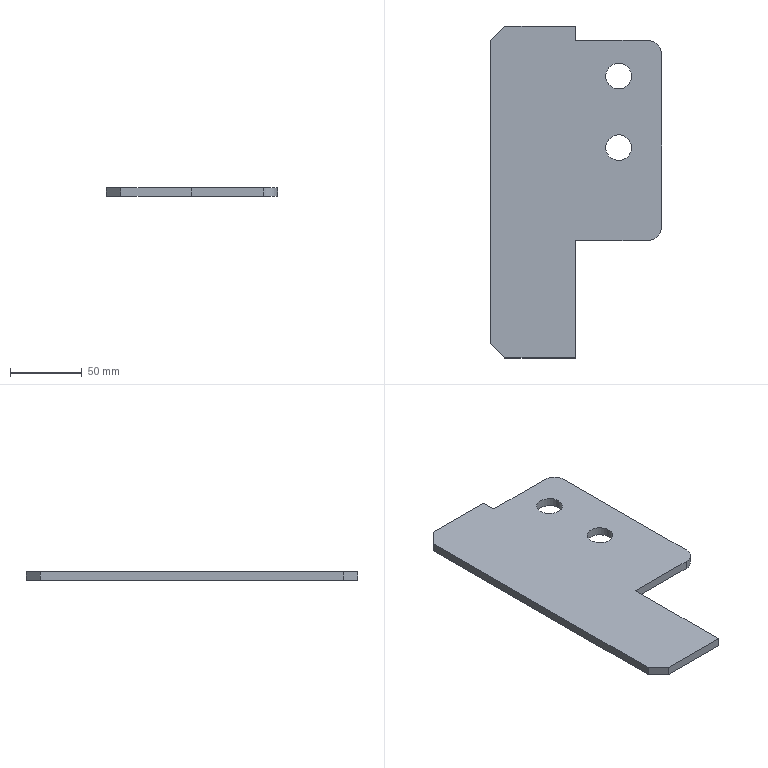Part | STEP file | PN_0034 channel connecting plate_Default<As Machined> | 1 solid | 16 faces | box 119.5 x 232 x 6 mm | volume 129313 mm3 | plane 12 | cylinder 4 | commonest cylinder face diameters 18 x2 20 x2
STEP:
#1=CARTESIAN_POINT('',(0.,0.,0.));
#2=DIRECTION('',(0.,0.,1.));
#3=DIRECTION('',(1.,0.,0.));
#4=AXIS2_PLACEMENT_3D('',#1,#2,#3);
#5=CARTESIAN_POINT('',(-19.75,-116.,6.));
#6=VERTEX_POINT('',#5);
#7=CARTESIAN_POINT('',(-19.75,-116.,0.));
#8=VERTEX_POINT('',#7);
#9=CARTESIAN_POINT('',(-19.75,-116.,6.));
#10=DIRECTION('',(0.,0.,-1.));
#11=VECTOR('',#10,1.);
#12=LINE('',#9,#11);
#13=CARTESIAN_POINT('',(-19.75,-116.,6.));
#14=DIRECTION('',(0.7071,0.7071,0.));
#15=DIRECTION('',(0.,0.,-1.));
#16=AXIS2_PLACEMENT_3D('',#13,#14,#15);
#17=PLANE('',#16);
#18=CARTESIAN_POINT('',(0.,0.));
#19=DIRECTION('',(1.,0.));
#20=VECTOR('',#19,1.);
#21=LINE('',#18,#20);
#22=(GEOMETRIC_REPRESENTATION_CONTEXT(2)PARAMETRIC_REPRESENTATION_CONTEXT()REPRESENTATION_CONTEXT('',''));
#23=DEFINITIONAL_REPRESENTATION('',(#21),#22);
#24=PCURVE('',#17,#23);
#25=CARTESIAN_POINT('',(-29.75,-116.,6.));
#26=DIRECTION('',(0.,1.,0.));
#27=DIRECTION('',(0.,0.,1.));
#28=AXIS2_PLACEMENT_3D('',#25,#26,#27);
#29=PLANE('',#28);
#30=CARTESIAN_POINT('',(0.,10.));
#31=DIRECTION('',(-1.,0.));
#32=VECTOR('',#31,1.);
#33=LINE('',#30,#32);
#34=(GEOMETRIC_REPRESENTATION_CONTEXT(2)PARAMETRIC_REPRESENTATION_CONTEXT()REPRESENTATION_CONTEXT('',''));
#35=DEFINITIONAL_REPRESENTATION('',(#33),#34);
#36=PCURVE('',#29,#35);
#37=SURFACE_CURVE('',#12,(#24,#36),.PCURVE_S1.);
#38=EDGE_CURVE('',#6,#8,#37,.T.);
#39=ORIENTED_EDGE('',*,*,#38,.F.);
#40=CARTESIAN_POINT('',(-29.75,-106.,6.));
#41=VERTEX_POINT('',#40);
#42=CARTESIAN_POINT('',(-67.875,-67.875,6.));
#43=DIRECTION('',(0.7071,-0.7071,0.));
#44=VECTOR('',#43,1.);
#45=LINE('',#42,#44);
#46=CARTESIAN_POINT('',(0.,68.059));
#47=DIRECTION('',(0.,-1.));
#48=VECTOR('',#47,1.);
#49=LINE('',#46,#48);
#50=(GEOMETRIC_REPRESENTATION_CONTEXT(2)PARAMETRIC_REPRESENTATION_CONTEXT()REPRESENTATION_CONTEXT('',''));
#51=DEFINITIONAL_REPRESENTATION('',(#49),#50);
#52=PCURVE('',#17,#51);
#53=CARTESIAN_POINT('',(0.,0.,6.));
#54=DIRECTION('',(0.,0.,1.));
#55=DIRECTION('',(1.,0.,0.));
#56=AXIS2_PLACEMENT_3D('',#53,#54,#55);
#57=PLANE('',#56);
#58=CARTESIAN_POINT('',(-67.875,-67.875));
#59=DIRECTION('',(0.7071,-0.7071));
#60=VECTOR('',#59,1.);
#61=LINE('',#58,#60);
#62=(GEOMETRIC_REPRESENTATION_CONTEXT(2)PARAMETRIC_REPRESENTATION_CONTEXT()REPRESENTATION_CONTEXT('',''));
#63=DEFINITIONAL_REPRESENTATION('',(#61),#62);
#64=PCURVE('',#57,#63);
#65=SURFACE_CURVE('',#45,(#52,#64),.PCURVE_S1.);
#66=EDGE_CURVE('',#41,#6,#65,.T.);
#67=ORIENTED_EDGE('',*,*,#66,.F.);
#68=CARTESIAN_POINT('',(-29.75,-106.,0.));
#69=VERTEX_POINT('',#68);
#70=CARTESIAN_POINT('',(-29.75,-106.,6.));
#71=DIRECTION('',(0.,0.,1.));
#72=VECTOR('',#71,1.);
#73=LINE('',#70,#72);
#74=CARTESIAN_POINT('',(0.,14.142));
#75=DIRECTION('',(-1.,0.));
#76=VECTOR('',#75,1.);
#77=LINE('',#74,#76);
#78=(GEOMETRIC_REPRESENTATION_CONTEXT(2)PARAMETRIC_REPRESENTATION_CONTEXT()REPRESENTATION_CONTEXT('',''));
#79=DEFINITIONAL_REPRESENTATION('',(#77),#78);
#80=PCURVE('',#17,#79);
#81=CARTESIAN_POINT('',(-29.75,116.,6.));
#82=DIRECTION('',(1.,0.,0.));
#83=DIRECTION('',(0.,0.,-1.));
#84=AXIS2_PLACEMENT_3D('',#81,#82,#83);
#85=PLANE('',#84);
#86=CARTESIAN_POINT('',(0.,-222.));
#87=DIRECTION('',(-1.,0.));
#88=VECTOR('',#87,1.);
#89=LINE('',#86,#88);
#90=(GEOMETRIC_REPRESENTATION_CONTEXT(2)PARAMETRIC_REPRESENTATION_CONTEXT()REPRESENTATION_CONTEXT('',''));
#91=DEFINITIONAL_REPRESENTATION('',(#89),#90);
#92=PCURVE('',#85,#91);
#93=SURFACE_CURVE('',#73,(#80,#92),.PCURVE_S1.);
#94=EDGE_CURVE('',#69,#41,#93,.T.);
#95=ORIENTED_EDGE('',*,*,#94,.F.);
#96=CARTESIAN_POINT('',(-19.75,-116.,0.));
#97=DIRECTION('',(-0.7071,0.7071,0.));
#98=VECTOR('',#97,1.);
#99=LINE('',#96,#98);
#100=CARTESIAN_POINT('',(6.,0.));
#101=DIRECTION('',(0.,1.));
#102=VECTOR('',#101,1.);
#103=LINE('',#100,#102);
#104=(GEOMETRIC_REPRESENTATION_CONTEXT(2)PARAMETRIC_REPRESENTATION_CONTEXT()REPRESENTATION_CONTEXT('',''));
#105=DEFINITIONAL_REPRESENTATION('',(#103),#104);
#106=PCURVE('',#17,#105);
#107=CARTESIAN_POINT('',(0.,0.,0.));
#108=DIRECTION('',(0.,0.,1.));
#109=DIRECTION('',(1.,0.,0.));
#110=AXIS2_PLACEMENT_3D('',#107,#108,#109);
#111=PLANE('',#110);
#112=CARTESIAN_POINT('',(-19.75,-116.));
#113=DIRECTION('',(-0.7071,0.7071));
#114=VECTOR('',#113,1.);
#115=LINE('',#112,#114);
#116=(GEOMETRIC_REPRESENTATION_CONTEXT(2)PARAMETRIC_REPRESENTATION_CONTEXT()REPRESENTATION_CONTEXT('',''));
#117=DEFINITIONAL_REPRESENTATION('',(#115),#116);
#118=PCURVE('',#111,#117);
#119=SURFACE_CURVE('',#99,(#106,#118),.PCURVE_S1.);
#120=EDGE_CURVE('',#8,#69,#119,.T.);
#121=ORIENTED_EDGE('',*,*,#120,.F.);
#122=EDGE_LOOP('',(#39,#67,#95,#121));
#123=FACE_BOUND('',#122,.T.);
#124=ADVANCED_FACE('',(#123),#17,.F.);
#125=CARTESIAN_POINT('',(-19.75,116.,0.));
#126=VERTEX_POINT('',#125);
#127=CARTESIAN_POINT('',(-19.75,116.,6.));
#128=VERTEX_POINT('',#127);
#129=CARTESIAN_POINT('',(-19.75,116.,6.));
#130=DIRECTION('',(0.,0.,1.));
#131=VECTOR('',#130,1.);
#132=LINE('',#129,#131);
#133=CARTESIAN_POINT('',(-19.75,116.,6.));
#134=DIRECTION('',(0.7071,-0.7071,0.));
#135=DIRECTION('',(0.,0.,1.));
#136=AXIS2_PLACEMENT_3D('',#133,#134,#135);
#137=PLANE('',#136);
#138=CARTESIAN_POINT('',(0.,0.));
#139=DIRECTION('',(1.,0.));
#140=VECTOR('',#139,1.);
#141=LINE('',#138,#140);
#142=(GEOMETRIC_REPRESENTATION_CONTEXT(2)PARAMETRIC_REPRESENTATION_CONTEXT()REPRESENTATION_CONTEXT('',''));
#143=DEFINITIONAL_REPRESENTATION('',(#141),#142);
#144=PCURVE('',#137,#143);
#145=CARTESIAN_POINT('',(-29.75,116.,6.));
#146=DIRECTION('',(0.,-1.,0.));
#147=DIRECTION('',(0.,0.,-1.));
#148=AXIS2_PLACEMENT_3D('',#145,#146,#147);
#149=PLANE('',#148);
#150=CARTESIAN_POINT('',(0.,10.));
#151=DIRECTION('',(-1.,0.));
#152=VECTOR('',#151,1.);
#153=LINE('',#150,#152);
#154=(GEOMETRIC_REPRESENTATION_CONTEXT(2)PARAMETRIC_REPRESENTATION_CONTEXT()REPRESENTATION_CONTEXT('',''));
#155=DEFINITIONAL_REPRESENTATION('',(#153),#154);
#156=PCURVE('',#149,#155);
#157=SURFACE_CURVE('',#132,(#144,#156),.PCURVE_S1.);
#158=EDGE_CURVE('',#126,#128,#157,.T.);
#159=ORIENTED_EDGE('',*,*,#158,.F.);
#160=CARTESIAN_POINT('',(-29.75,106.,0.));
#161=VERTEX_POINT('',#160);
#162=CARTESIAN_POINT('',(-19.75,116.,0.));
#163=DIRECTION('',(0.7071,0.7071,0.));
#164=VECTOR('',#163,1.);
#165=LINE('',#162,#164);
#166=CARTESIAN_POINT('',(-6.,0.));
#167=DIRECTION('',(0.,-1.));
#168=VECTOR('',#167,1.);
#169=LINE('',#166,#168);
#170=(GEOMETRIC_REPRESENTATION_CONTEXT(2)PARAMETRIC_REPRESENTATION_CONTEXT()REPRESENTATION_CONTEXT('',''));
#171=DEFINITIONAL_REPRESENTATION('',(#169),#170);
#172=PCURVE('',#137,#171);
#173=CARTESIAN_POINT('',(-19.75,116.));
#174=DIRECTION('',(0.7071,0.7071));
#175=VECTOR('',#174,1.);
#176=LINE('',#173,#175);
#177=(GEOMETRIC_REPRESENTATION_CONTEXT(2)PARAMETRIC_REPRESENTATION_CONTEXT()REPRESENTATION_CONTEXT('',''));
#178=DEFINITIONAL_REPRESENTATION('',(#176),#177);
#179=PCURVE('',#111,#178);
#180=SURFACE_CURVE('',#165,(#172,#179),.PCURVE_S1.);
#181=EDGE_CURVE('',#161,#126,#180,.T.);
#182=ORIENTED_EDGE('',*,*,#181,.F.);
#183=CARTESIAN_POINT('',(-29.75,106.,6.));
#184=VERTEX_POINT('',#183);
#185=CARTESIAN_POINT('',(-29.75,106.,6.));
#186=DIRECTION('',(0.,0.,-1.));
#187=VECTOR('',#186,1.);
#188=LINE('',#185,#187);
#189=CARTESIAN_POINT('',(0.,14.142));
#190=DIRECTION('',(-1.,0.));
#191=VECTOR('',#190,1.);
#192=LINE('',#189,#191);
#193=(GEOMETRIC_REPRESENTATION_CONTEXT(2)PARAMETRIC_REPRESENTATION_CONTEXT()REPRESENTATION_CONTEXT('',''));
#194=DEFINITIONAL_REPRESENTATION('',(#192),#193);
#195=PCURVE('',#137,#194);
#196=CARTESIAN_POINT('',(0.,-10.));
#197=DIRECTION('',(1.,0.));
#198=VECTOR('',#197,1.);
#199=LINE('',#196,#198);
#200=(GEOMETRIC_REPRESENTATION_CONTEXT(2)PARAMETRIC_REPRESENTATION_CONTEXT()REPRESENTATION_CONTEXT('',''));
#201=DEFINITIONAL_REPRESENTATION('',(#199),#200);
#202=PCURVE('',#85,#201);
#203=SURFACE_CURVE('',#188,(#195,#202),.PCURVE_S1.);
#204=EDGE_CURVE('',#184,#161,#203,.T.);
#205=ORIENTED_EDGE('',*,*,#204,.F.);
#206=CARTESIAN_POINT('',(-67.875,67.875,6.));
#207=DIRECTION('',(-0.7071,-0.7071,0.));
#208=VECTOR('',#207,1.);
#209=LINE('',#206,#208);
#210=CARTESIAN_POINT('',(0.,68.059));
#211=DIRECTION('',(0.,1.));
#212=VECTOR('',#211,1.);
#213=LINE('',#210,#212);
#214=(GEOMETRIC_REPRESENTATION_CONTEXT(2)PARAMETRIC_REPRESENTATION_CONTEXT()REPRESENTATION_CONTEXT('',''));
#215=DEFINITIONAL_REPRESENTATION('',(#213),#214);
#216=PCURVE('',#137,#215);
#217=CARTESIAN_POINT('',(-67.875,67.875));
#218=DIRECTION('',(-0.7071,-0.7071));
#219=VECTOR('',#218,1.);
#220=LINE('',#217,#219);
#221=(GEOMETRIC_REPRESENTATION_CONTEXT(2)PARAMETRIC_REPRESENTATION_CONTEXT()REPRESENTATION_CONTEXT('',''));
#222=DEFINITIONAL_REPRESENTATION('',(#220),#221);
#223=PCURVE('',#57,#222);
#224=SURFACE_CURVE('',#209,(#216,#223),.PCURVE_S1.);
#225=EDGE_CURVE('',#128,#184,#224,.T.);
#226=ORIENTED_EDGE('',*,*,#225,.F.);
#227=EDGE_LOOP('',(#159,#182,#205,#226));
#228=FACE_BOUND('',#227,.T.);
#229=ADVANCED_FACE('',(#228),#137,.F.);
#230=CARTESIAN_POINT('',(29.75,-116.,0.));
#231=VERTEX_POINT('',#230);
#232=CARTESIAN_POINT('',(29.75,-34.,0.));
#233=VERTEX_POINT('',#232);
#234=CARTESIAN_POINT('',(29.75,-34.,0.));
#235=DIRECTION('',(0.,1.,0.));
#236=VECTOR('',#235,1.);
#237=LINE('',#234,#236);
#238=CARTESIAN_POINT('',(29.75,-34.,6.));
#239=DIRECTION('',(-1.,0.,0.));
#240=DIRECTION('',(0.,-1.,0.));
#241=AXIS2_PLACEMENT_3D('',#238,#239,#240);
#242=PLANE('',#241);
#243=CARTESIAN_POINT('',(0.,-6.));
#244=DIRECTION('',(-1.,0.));
#245=VECTOR('',#244,1.);
#246=LINE('',#243,#245);
#247=(GEOMETRIC_REPRESENTATION_CONTEXT(2)PARAMETRIC_REPRESENTATION_CONTEXT()REPRESENTATION_CONTEXT('',''));
#248=DEFINITIONAL_REPRESENTATION('',(#246),#247);
#249=PCURVE('',#242,#248);
#250=CARTESIAN_POINT('',(29.75,-34.));
#251=DIRECTION('',(0.,1.));
#252=VECTOR('',#251,1.);
#253=LINE('',#250,#252);
#254=(GEOMETRIC_REPRESENTATION_CONTEXT(2)PARAMETRIC_REPRESENTATION_CONTEXT()REPRESENTATION_CONTEXT('',''));
#255=DEFINITIONAL_REPRESENTATION('',(#253),#254);
#256=PCURVE('',#111,#255);
#257=SURFACE_CURVE('',#237,(#249,#256),.PCURVE_S1.);
#258=EDGE_CURVE('',#231,#233,#257,.T.);
#259=ORIENTED_EDGE('',*,*,#258,.T.);
#260=CARTESIAN_POINT('',(29.75,-34.,6.));
#261=VERTEX_POINT('',#260);
#262=CARTESIAN_POINT('',(29.75,-34.,6.));
#263=DIRECTION('',(0.,0.,-1.));
#264=VECTOR('',#263,1.);
#265=LINE('',#262,#264);
#266=CARTESIAN_POINT('',(0.,0.));
#267=DIRECTION('',(0.,-1.));
#268=VECTOR('',#267,1.);
#269=LINE('',#266,#268);
#270=(GEOMETRIC_REPRESENTATION_CONTEXT(2)PARAMETRIC_REPRESENTATION_CONTEXT()REPRESENTATION_CONTEXT('',''));
#271=DEFINITIONAL_REPRESENTATION('',(#269),#270);
#272=PCURVE('',#242,#271);
#273=CARTESIAN_POINT('',(89.75,-34.,6.));
#274=DIRECTION('',(0.,1.,0.));
#275=DIRECTION('',(-1.,0.,0.));
#276=AXIS2_PLACEMENT_3D('',#273,#274,#275);
#277=PLANE('',#276);
#278=CARTESIAN_POINT('',(60.,0.));
#279=DIRECTION('',(0.,-1.));
#280=VECTOR('',#279,1.);
#281=LINE('',#278,#280);
#282=(GEOMETRIC_REPRESENTATION_CONTEXT(2)PARAMETRIC_REPRESENTATION_CONTEXT()REPRESENTATION_CONTEXT('',''));
#283=DEFINITIONAL_REPRESENTATION('',(#281),#282);
#284=PCURVE('',#277,#283);
#285=SURFACE_CURVE('',#265,(#272,#284),.PCURVE_S1.);
#286=EDGE_CURVE('',#261,#233,#285,.T.);
#287=ORIENTED_EDGE('',*,*,#286,.F.);
#288=CARTESIAN_POINT('',(29.75,-116.,6.));
#289=VERTEX_POINT('',#288);
#290=CARTESIAN_POINT('',(29.75,-34.,6.));
#291=DIRECTION('',(0.,1.,0.));
#292=VECTOR('',#291,1.);
#293=LINE('',#290,#292);
#294=CARTESIAN_POINT('',(0.,0.));
#295=DIRECTION('',(-1.,0.));
#296=VECTOR('',#295,1.);
#297=LINE('',#294,#296);
#298=(GEOMETRIC_REPRESENTATION_CONTEXT(2)PARAMETRIC_REPRESENTATION_CONTEXT()REPRESENTATION_CONTEXT('',''));
#299=DEFINITIONAL_REPRESENTATION('',(#297),#298);
#300=PCURVE('',#242,#299);
#301=CARTESIAN_POINT('',(29.75,-34.));
#302=DIRECTION('',(0.,1.));
#303=VECTOR('',#302,1.);
#304=LINE('',#301,#303);
#305=(GEOMETRIC_REPRESENTATION_CONTEXT(2)PARAMETRIC_REPRESENTATION_CONTEXT()REPRESENTATION_CONTEXT('',''));
#306=DEFINITIONAL_REPRESENTATION('',(#304),#305);
#307=PCURVE('',#57,#306);
#308=SURFACE_CURVE('',#293,(#300,#307),.PCURVE_S1.);
#309=EDGE_CURVE('',#289,#261,#308,.T.);
#310=ORIENTED_EDGE('',*,*,#309,.F.);
#311=CARTESIAN_POINT('',(29.75,-116.,6.));
#312=DIRECTION('',(0.,0.,-1.));
#313=VECTOR('',#312,1.);
#314=LINE('',#311,#313);
#315=CARTESIAN_POINT('',(82.,0.));
#316=DIRECTION('',(0.,-1.));
#317=VECTOR('',#316,1.);
#318=LINE('',#315,#317);
#319=(GEOMETRIC_REPRESENTATION_CONTEXT(2)PARAMETRIC_REPRESENTATION_CONTEXT()REPRESENTATION_CONTEXT('',''));
#320=DEFINITIONAL_REPRESENTATION('',(#318),#319);
#321=PCURVE('',#242,#320);
#322=CARTESIAN_POINT('',(0.,59.5));
#323=DIRECTION('',(-1.,0.));
#324=VECTOR('',#323,1.);
#325=LINE('',#322,#324);
#326=(GEOMETRIC_REPRESENTATION_CONTEXT(2)PARAMETRIC_REPRESENTATION_CONTEXT()REPRESENTATION_CONTEXT('',''));
#327=DEFINITIONAL_REPRESENTATION('',(#325),#326);
#328=PCURVE('',#29,#327);
#329=SURFACE_CURVE('',#314,(#321,#328),.PCURVE_S1.);
#330=EDGE_CURVE('',#289,#231,#329,.T.);
#331=ORIENTED_EDGE('',*,*,#330,.T.);
#332=EDGE_LOOP('',(#259,#287,#310,#331));
#333=FACE_BOUND('',#332,.T.);
#334=ADVANCED_FACE('',(#333),#242,.F.);
#335=CARTESIAN_POINT('',(79.75,-34.,0.));
#336=VERTEX_POINT('',#335);
#337=CARTESIAN_POINT('',(89.75,-34.,0.));
#338=DIRECTION('',(1.,0.,0.));
#339=VECTOR('',#338,1.);
#340=LINE('',#337,#339);
#341=CARTESIAN_POINT('',(0.,-6.));
#342=DIRECTION('',(-1.,0.));
#343=VECTOR('',#342,1.);
#344=LINE('',#341,#343);
#345=(GEOMETRIC_REPRESENTATION_CONTEXT(2)PARAMETRIC_REPRESENTATION_CONTEXT()REPRESENTATION_CONTEXT('',''));
#346=DEFINITIONAL_REPRESENTATION('',(#344),#345);
#347=PCURVE('',#277,#346);
#348=CARTESIAN_POINT('',(89.75,-34.));
#349=DIRECTION('',(1.,0.));
#350=VECTOR('',#349,1.);
#351=LINE('',#348,#350);
#352=(GEOMETRIC_REPRESENTATION_CONTEXT(2)PARAMETRIC_REPRESENTATION_CONTEXT()REPRESENTATION_CONTEXT('',''));
#353=DEFINITIONAL_REPRESENTATION('',(#351),#352);
#354=PCURVE('',#111,#353);
#355=SURFACE_CURVE('',#340,(#347,#354),.PCURVE_S1.);
#356=EDGE_CURVE('',#233,#336,#355,.T.);
#357=ORIENTED_EDGE('',*,*,#356,.T.);
#358=CARTESIAN_POINT('',(79.75,-34.,6.));
#359=VERTEX_POINT('',#358);
#360=CARTESIAN_POINT('',(79.75,-34.,6.));
#361=DIRECTION('',(0.,0.,1.));
#362=VECTOR('',#361,1.);
#363=LINE('',#360,#362);
#364=CARTESIAN_POINT('',(10.,0.));
#365=DIRECTION('',(0.,1.));
#366=VECTOR('',#365,1.);
#367=LINE('',#364,#366);
#368=(GEOMETRIC_REPRESENTATION_CONTEXT(2)PARAMETRIC_REPRESENTATION_CONTEXT()REPRESENTATION_CONTEXT('',''));
#369=DEFINITIONAL_REPRESENTATION('',(#367),#368);
#370=PCURVE('',#277,#369);
#371=CARTESIAN_POINT('',(79.75,-24.,6.));
#372=DIRECTION('',(0.,0.,-1.));
#373=DIRECTION('',(-1.,0.,0.));
#374=AXIS2_PLACEMENT_3D('',#371,#372,#373);
#375=CYLINDRICAL_SURFACE('',#374,10.);
#376=CARTESIAN_POINT('',(4.712,0.));
#377=DIRECTION('',(0.,-1.));
#378=VECTOR('',#377,1.);
#379=LINE('',#376,#378);
#380=(GEOMETRIC_REPRESENTATION_CONTEXT(2)PARAMETRIC_REPRESENTATION_CONTEXT()REPRESENTATION_CONTEXT('',''));
#381=DEFINITIONAL_REPRESENTATION('',(#379),#380);
#382=PCURVE('',#375,#381);
#383=SURFACE_CURVE('',#363,(#370,#382),.PCURVE_S1.);
#384=EDGE_CURVE('',#336,#359,#383,.T.);
#385=ORIENTED_EDGE('',*,*,#384,.T.);
#386=CARTESIAN_POINT('',(89.75,-34.,6.));
#387=DIRECTION('',(1.,0.,0.));
#388=VECTOR('',#387,1.);
#389=LINE('',#386,#388);
#390=CARTESIAN_POINT('',(0.,0.));
#391=DIRECTION('',(-1.,0.));
#392=VECTOR('',#391,1.);
#393=LINE('',#390,#392);
#394=(GEOMETRIC_REPRESENTATION_CONTEXT(2)PARAMETRIC_REPRESENTATION_CONTEXT()REPRESENTATION_CONTEXT('',''));
#395=DEFINITIONAL_REPRESENTATION('',(#393),#394);
#396=PCURVE('',#277,#395);
#397=CARTESIAN_POINT('',(89.75,-34.));
#398=DIRECTION('',(1.,0.));
#399=VECTOR('',#398,1.);
#400=LINE('',#397,#399);
#401=(GEOMETRIC_REPRESENTATION_CONTEXT(2)PARAMETRIC_REPRESENTATION_CONTEXT()REPRESENTATION_CONTEXT('',''));
#402=DEFINITIONAL_REPRESENTATION('',(#400),#401);
#403=PCURVE('',#57,#402);
#404=SURFACE_CURVE('',#389,(#396,#403),.PCURVE_S1.);
#405=EDGE_CURVE('',#261,#359,#404,.T.);
#406=ORIENTED_EDGE('',*,*,#405,.F.);
#407=ORIENTED_EDGE('',*,*,#286,.T.);
#408=EDGE_LOOP('',(#357,#385,#406,#407));
#409=FACE_BOUND('',#408,.T.);
#410=ADVANCED_FACE('',(#409),#277,.F.);
#411=CARTESIAN_POINT('',(89.75,-24.,6.));
#412=VERTEX_POINT('',#411);
#413=CARTESIAN_POINT('',(89.75,96.,6.));
#414=VERTEX_POINT('',#413);
#415=CARTESIAN_POINT('',(89.75,106.,6.));
#416=DIRECTION('',(0.,1.,0.));
#417=VECTOR('',#416,1.);
#418=LINE('',#415,#417);
#419=CARTESIAN_POINT('',(89.75,106.,6.));
#420=DIRECTION('',(-1.,0.,0.));
#421=DIRECTION('',(0.,-1.,0.));
#422=AXIS2_PLACEMENT_3D('',#419,#420,#421);
#423=PLANE('',#422);
#424=CARTESIAN_POINT('',(0.,0.));
#425=DIRECTION('',(-1.,0.));
#426=VECTOR('',#425,1.);
#427=LINE('',#424,#426);
#428=(GEOMETRIC_REPRESENTATION_CONTEXT(2)PARAMETRIC_REPRESENTATION_CONTEXT()REPRESENTATION_CONTEXT('',''));
#429=DEFINITIONAL_REPRESENTATION('',(#427),#428);
#430=PCURVE('',#423,#429);
#431=CARTESIAN_POINT('',(89.75,106.));
#432=DIRECTION('',(0.,1.));
#433=VECTOR('',#432,1.);
#434=LINE('',#431,#433);
#435=(GEOMETRIC_REPRESENTATION_CONTEXT(2)PARAMETRIC_REPRESENTATION_CONTEXT()REPRESENTATION_CONTEXT('',''));
#436=DEFINITIONAL_REPRESENTATION('',(#434),#435);
#437=PCURVE('',#57,#436);
#438=SURFACE_CURVE('',#418,(#430,#437),.PCURVE_S1.);
#439=EDGE_CURVE('',#412,#414,#438,.T.);
#440=ORIENTED_EDGE('',*,*,#439,.F.);
#441=CARTESIAN_POINT('',(89.75,-24.,0.));
#442=VERTEX_POINT('',#441);
#443=CARTESIAN_POINT('',(89.75,-24.,6.));
#444=DIRECTION('',(0.,0.,-1.));
#445=VECTOR('',#444,1.);
#446=LINE('',#443,#445);
#447=CARTESIAN_POINT('',(130.,0.));
#448=DIRECTION('',(0.,-1.));
#449=VECTOR('',#448,1.);
#450=LINE('',#447,#449);
#451=(GEOMETRIC_REPRESENTATION_CONTEXT(2)PARAMETRIC_REPRESENTATION_CONTEXT()REPRESENTATION_CONTEXT('',''));
#452=DEFINITIONAL_REPRESENTATION('',(#450),#451);
#453=PCURVE('',#423,#452);
#454=CARTESIAN_POINT('',(3.142,0.));
#455=DIRECTION('',(0.,1.));
#456=VECTOR('',#455,1.);
#457=LINE('',#454,#456);
#458=(GEOMETRIC_REPRESENTATION_CONTEXT(2)PARAMETRIC_REPRESENTATION_CONTEXT()REPRESENTATION_CONTEXT('',''));
#459=DEFINITIONAL_REPRESENTATION('',(#457),#458);
#460=PCURVE('',#375,#459);
#461=SURFACE_CURVE('',#446,(#453,#460),.PCURVE_S1.);
#462=EDGE_CURVE('',#412,#442,#461,.T.);
#463=ORIENTED_EDGE('',*,*,#462,.T.);
#464=CARTESIAN_POINT('',(89.75,96.,0.));
#465=VERTEX_POINT('',#464);
#466=CARTESIAN_POINT('',(89.75,106.,0.));
#467=DIRECTION('',(0.,1.,0.));
#468=VECTOR('',#467,1.);
#469=LINE('',#466,#468);
#470=CARTESIAN_POINT('',(0.,-6.));
#471=DIRECTION('',(-1.,0.));
#472=VECTOR('',#471,1.);
#473=LINE('',#470,#472);
#474=(GEOMETRIC_REPRESENTATION_CONTEXT(2)PARAMETRIC_REPRESENTATION_CONTEXT()REPRESENTATION_CONTEXT('',''));
#475=DEFINITIONAL_REPRESENTATION('',(#473),#474);
#476=PCURVE('',#423,#475);
#477=CARTESIAN_POINT('',(89.75,106.));
#478=DIRECTION('',(0.,1.));
#479=VECTOR('',#478,1.);
#480=LINE('',#477,#479);
#481=(GEOMETRIC_REPRESENTATION_CONTEXT(2)PARAMETRIC_REPRESENTATION_CONTEXT()REPRESENTATION_CONTEXT('',''));
#482=DEFINITIONAL_REPRESENTATION('',(#480),#481);
#483=PCURVE('',#111,#482);
#484=SURFACE_CURVE('',#469,(#476,#483),.PCURVE_S1.);
#485=EDGE_CURVE('',#442,#465,#484,.T.);
#486=ORIENTED_EDGE('',*,*,#485,.T.);
#487=CARTESIAN_POINT('',(89.75,96.,6.));
#488=DIRECTION('',(0.,0.,1.));
#489=VECTOR('',#488,1.);
#490=LINE('',#487,#489);
#491=CARTESIAN_POINT('',(10.,0.));
#492=DIRECTION('',(0.,1.));
#493=VECTOR('',#492,1.);
#494=LINE('',#491,#493);
#495=(GEOMETRIC_REPRESENTATION_CONTEXT(2)PARAMETRIC_REPRESENTATION_CONTEXT()REPRESENTATION_CONTEXT('',''));
#496=DEFINITIONAL_REPRESENTATION('',(#494),#495);
#497=PCURVE('',#423,#496);
#498=CARTESIAN_POINT('',(79.75,96.,6.));
#499=DIRECTION('',(0.,0.,-1.));
#500=DIRECTION('',(-1.,0.,0.));
#501=AXIS2_PLACEMENT_3D('',#498,#499,#500);
#502=CYLINDRICAL_SURFACE('',#501,10.);
#503=CARTESIAN_POINT('',(3.142,0.));
#504=DIRECTION('',(0.,-1.));
#505=VECTOR('',#504,1.);
#506=LINE('',#503,#505);
#507=(GEOMETRIC_REPRESENTATION_CONTEXT(2)PARAMETRIC_REPRESENTATION_CONTEXT()REPRESENTATION_CONTEXT('',''));
#508=DEFINITIONAL_REPRESENTATION('',(#506),#507);
#509=PCURVE('',#502,#508);
#510=SURFACE_CURVE('',#490,(#497,#509),.PCURVE_S1.);
#511=EDGE_CURVE('',#465,#414,#510,.T.);
#512=ORIENTED_EDGE('',*,*,#511,.T.);
#513=EDGE_LOOP('',(#440,#463,#486,#512));
#514=FACE_BOUND('',#513,.T.);
#515=ADVANCED_FACE('',(#514),#423,.F.);
#516=CARTESIAN_POINT('',(79.75,106.,6.));
#517=VERTEX_POINT('',#516);
#518=CARTESIAN_POINT('',(29.75,106.,6.));
#519=VERTEX_POINT('',#518);
#520=CARTESIAN_POINT('',(29.75,106.,6.));
#521=DIRECTION('',(-1.,0.,0.));
#522=VECTOR('',#521,1.);
#523=LINE('',#520,#522);
#524=CARTESIAN_POINT('',(29.75,106.,6.));
#525=DIRECTION('',(0.,-1.,0.));
#526=DIRECTION('',(0.,0.,-1.));
#527=AXIS2_PLACEMENT_3D('',#524,#525,#526);
#528=PLANE('',#527);
#529=CARTESIAN_POINT('',(0.,0.));
#530=DIRECTION('',(0.,-1.));
#531=VECTOR('',#530,1.);
#532=LINE('',#529,#531);
#533=(GEOMETRIC_REPRESENTATION_CONTEXT(2)PARAMETRIC_REPRESENTATION_CONTEXT()REPRESENTATION_CONTEXT('',''));
#534=DEFINITIONAL_REPRESENTATION('',(#532),#533);
#535=PCURVE('',#528,#534);
#536=CARTESIAN_POINT('',(29.75,106.));
#537=DIRECTION('',(-1.,0.));
#538=VECTOR('',#537,1.);
#539=LINE('',#536,#538);
#540=(GEOMETRIC_REPRESENTATION_CONTEXT(2)PARAMETRIC_REPRESENTATION_CONTEXT()REPRESENTATION_CONTEXT('',''));
#541=DEFINITIONAL_REPRESENTATION('',(#539),#540);
#542=PCURVE('',#57,#541);
#543=SURFACE_CURVE('',#523,(#535,#542),.PCURVE_S1.);
#544=EDGE_CURVE('',#517,#519,#543,.T.);
#545=ORIENTED_EDGE('',*,*,#544,.F.);
#546=CARTESIAN_POINT('',(79.75,106.,0.));
#547=VERTEX_POINT('',#546);
#548=CARTESIAN_POINT('',(79.75,106.,6.));
#549=DIRECTION('',(0.,0.,-1.));
#550=VECTOR('',#549,1.);
#551=LINE('',#548,#550);
#552=CARTESIAN_POINT('',(0.,50.));
#553=DIRECTION('',(1.,0.));
#554=VECTOR('',#553,1.);
#555=LINE('',#552,#554);
#556=(GEOMETRIC_REPRESENTATION_CONTEXT(2)PARAMETRIC_REPRESENTATION_CONTEXT()REPRESENTATION_CONTEXT('',''));
#557=DEFINITIONAL_REPRESENTATION('',(#555),#556);
#558=PCURVE('',#528,#557);
#559=CARTESIAN_POINT('',(1.571,0.));
#560=DIRECTION('',(0.,1.));
#561=VECTOR('',#560,1.);
#562=LINE('',#559,#561);
#563=(GEOMETRIC_REPRESENTATION_CONTEXT(2)PARAMETRIC_REPRESENTATION_CONTEXT()REPRESENTATION_CONTEXT('',''));
#564=DEFINITIONAL_REPRESENTATION('',(#562),#563);
#565=PCURVE('',#502,#564);
#566=SURFACE_CURVE('',#551,(#558,#565),.PCURVE_S1.);
#567=EDGE_CURVE('',#517,#547,#566,.T.);
#568=ORIENTED_EDGE('',*,*,#567,.T.);
#569=CARTESIAN_POINT('',(29.75,106.,0.));
#570=VERTEX_POINT('',#569);
#571=CARTESIAN_POINT('',(29.75,106.,0.));
#572=DIRECTION('',(-1.,0.,0.));
#573=VECTOR('',#572,1.);
#574=LINE('',#571,#573);
#575=CARTESIAN_POINT('',(6.,0.));
#576=DIRECTION('',(0.,-1.));
#577=VECTOR('',#576,1.);
#578=LINE('',#575,#577);
#579=(GEOMETRIC_REPRESENTATION_CONTEXT(2)PARAMETRIC_REPRESENTATION_CONTEXT()REPRESENTATION_CONTEXT('',''));
#580=DEFINITIONAL_REPRESENTATION('',(#578),#579);
#581=PCURVE('',#528,#580);
#582=CARTESIAN_POINT('',(29.75,106.));
#583=DIRECTION('',(-1.,0.));
#584=VECTOR('',#583,1.);
#585=LINE('',#582,#584);
#586=(GEOMETRIC_REPRESENTATION_CONTEXT(2)PARAMETRIC_REPRESENTATION_CONTEXT()REPRESENTATION_CONTEXT('',''));
#587=DEFINITIONAL_REPRESENTATION('',(#585),#586);
#588=PCURVE('',#111,#587);
#589=SURFACE_CURVE('',#574,(#581,#588),.PCURVE_S1.);
#590=EDGE_CURVE('',#547,#570,#589,.T.);
#591=ORIENTED_EDGE('',*,*,#590,.T.);
#592=CARTESIAN_POINT('',(29.75,106.,6.));
#593=DIRECTION('',(0.,0.,-1.));
#594=VECTOR('',#593,1.);
#595=LINE('',#592,#594);
#596=CARTESIAN_POINT('',(0.,0.));
#597=DIRECTION('',(1.,0.));
#598=VECTOR('',#597,1.);
#599=LINE('',#596,#598);
#600=(GEOMETRIC_REPRESENTATION_CONTEXT(2)PARAMETRIC_REPRESENTATION_CONTEXT()REPRESENTATION_CONTEXT('',''));
#601=DEFINITIONAL_REPRESENTATION('',(#599),#600);
#602=PCURVE('',#528,#601);
#603=CARTESIAN_POINT('',(29.75,116.,6.));
#604=DIRECTION('',(-1.,0.,0.));
#605=DIRECTION('',(0.,0.,1.));
#606=AXIS2_PLACEMENT_3D('',#603,#604,#605);
#607=PLANE('',#606);
#608=CARTESIAN_POINT('',(0.,-10.));
#609=DIRECTION('',(-1.,0.));
#610=VECTOR('',#609,1.);
#611=LINE('',#608,#610);
#612=(GEOMETRIC_REPRESENTATION_CONTEXT(2)PARAMETRIC_REPRESENTATION_CONTEXT()REPRESENTATION_CONTEXT('',''));
#613=DEFINITIONAL_REPRESENTATION('',(#611),#612);
#614=PCURVE('',#607,#613);
#615=SURFACE_CURVE('',#595,(#602,#614),.PCURVE_S1.);
#616=EDGE_CURVE('',#519,#570,#615,.T.);
#617=ORIENTED_EDGE('',*,*,#616,.F.);
#618=EDGE_LOOP('',(#545,#568,#591,#617));
#619=FACE_BOUND('',#618,.T.);
#620=ADVANCED_FACE('',(#619),#528,.F.);
#621=CARTESIAN_POINT('',(29.75,116.,0.));
#622=VERTEX_POINT('',#621);
#623=CARTESIAN_POINT('',(29.75,116.,0.));
#624=DIRECTION('',(0.,1.,0.));
#625=VECTOR('',#624,1.);
#626=LINE('',#623,#625);
#627=CARTESIAN_POINT('',(-6.,0.));
#628=DIRECTION('',(0.,1.));
#629=VECTOR('',#628,1.);
#630=LINE('',#627,#629);
#631=(GEOMETRIC_REPRESENTATION_CONTEXT(2)PARAMETRIC_REPRESENTATION_CONTEXT()REPRESENTATION_CONTEXT('',''));
#632=DEFINITIONAL_REPRESENTATION('',(#630),#631);
#633=PCURVE('',#607,#632);
#634=CARTESIAN_POINT('',(29.75,116.));
#635=DIRECTION('',(0.,1.));
#636=VECTOR('',#635,1.);
#637=LINE('',#634,#636);
#638=(GEOMETRIC_REPRESENTATION_CONTEXT(2)PARAMETRIC_REPRESENTATION_CONTEXT()REPRESENTATION_CONTEXT('',''));
#639=DEFINITIONAL_REPRESENTATION('',(#637),#638);
#640=PCURVE('',#111,#639);
#641=SURFACE_CURVE('',#626,(#633,#640),.PCURVE_S1.);
#642=EDGE_CURVE('',#570,#622,#641,.T.);
#643=ORIENTED_EDGE('',*,*,#642,.T.);
#644=CARTESIAN_POINT('',(29.75,116.,6.));
#645=VERTEX_POINT('',#644);
#646=CARTESIAN_POINT('',(29.75,116.,6.));
#647=DIRECTION('',(0.,0.,-1.));
#648=VECTOR('',#647,1.);
#649=LINE('',#646,#648);
#650=CARTESIAN_POINT('',(0.,0.));
#651=DIRECTION('',(-1.,0.));
#652=VECTOR('',#651,1.);
#653=LINE('',#650,#652);
#654=(GEOMETRIC_REPRESENTATION_CONTEXT(2)PARAMETRIC_REPRESENTATION_CONTEXT()REPRESENTATION_CONTEXT('',''));
#655=DEFINITIONAL_REPRESENTATION('',(#653),#654);
#656=PCURVE('',#607,#655);
#657=CARTESIAN_POINT('',(0.,59.5));
#658=DIRECTION('',(1.,0.));
#659=VECTOR('',#658,1.);
#660=LINE('',#657,#659);
#661=(GEOMETRIC_REPRESENTATION_CONTEXT(2)PARAMETRIC_REPRESENTATION_CONTEXT()REPRESENTATION_CONTEXT('',''));
#662=DEFINITIONAL_REPRESENTATION('',(#660),#661);
#663=PCURVE('',#149,#662);
#664=SURFACE_CURVE('',#649,(#656,#663),.PCURVE_S1.);
#665=EDGE_CURVE('',#645,#622,#664,.T.);
#666=ORIENTED_EDGE('',*,*,#665,.F.);
#667=CARTESIAN_POINT('',(29.75,116.,6.));
#668=DIRECTION('',(0.,1.,0.));
#669=VECTOR('',#668,1.);
#670=LINE('',#667,#669);
#671=CARTESIAN_POINT('',(0.,0.));
#672=DIRECTION('',(0.,1.));
#673=VECTOR('',#672,1.);
#674=LINE('',#671,#673);
#675=(GEOMETRIC_REPRESENTATION_CONTEXT(2)PARAMETRIC_REPRESENTATION_CONTEXT()REPRESENTATION_CONTEXT('',''));
#676=DEFINITIONAL_REPRESENTATION('',(#674),#675);
#677=PCURVE('',#607,#676);
#678=CARTESIAN_POINT('',(29.75,116.));
#679=DIRECTION('',(0.,1.));
#680=VECTOR('',#679,1.);
#681=LINE('',#678,#680);
#682=(GEOMETRIC_REPRESENTATION_CONTEXT(2)PARAMETRIC_REPRESENTATION_CONTEXT()REPRESENTATION_CONTEXT('',''));
#683=DEFINITIONAL_REPRESENTATION('',(#681),#682);
#684=PCURVE('',#57,#683);
#685=SURFACE_CURVE('',#670,(#677,#684),.PCURVE_S1.);
#686=EDGE_CURVE('',#519,#645,#685,.T.);
#687=ORIENTED_EDGE('',*,*,#686,.F.);
#688=ORIENTED_EDGE('',*,*,#616,.T.);
#689=EDGE_LOOP('',(#643,#666,#687,#688));
#690=FACE_BOUND('',#689,.T.);
#691=ADVANCED_FACE('',(#690),#607,.F.);
#692=CARTESIAN_POINT('',(-29.75,116.,0.));
#693=DIRECTION('',(-1.,0.,0.));
#694=VECTOR('',#693,1.);
#695=LINE('',#692,#694);
#696=CARTESIAN_POINT('',(6.,0.));
#697=DIRECTION('',(0.,-1.));
#698=VECTOR('',#697,1.);
#699=LINE('',#696,#698);
#700=(GEOMETRIC_REPRESENTATION_CONTEXT(2)PARAMETRIC_REPRESENTATION_CONTEXT()REPRESENTATION_CONTEXT('',''));
#701=DEFINITIONAL_REPRESENTATION('',(#699),#700);
#702=PCURVE('',#149,#701);
#703=CARTESIAN_POINT('',(-29.75,116.));
#704=DIRECTION('',(-1.,0.));
#705=VECTOR('',#704,1.);
#706=LINE('',#703,#705);
#707=(GEOMETRIC_REPRESENTATION_CONTEXT(2)PARAMETRIC_REPRESENTATION_CONTEXT()REPRESENTATION_CONTEXT('',''));
#708=DEFINITIONAL_REPRESENTATION('',(#706),#707);
#709=PCURVE('',#111,#708);
#710=SURFACE_CURVE('',#695,(#702,#709),.PCURVE_S1.);
#711=EDGE_CURVE('',#622,#126,#710,.T.);
#712=ORIENTED_EDGE('',*,*,#711,.T.);
#713=ORIENTED_EDGE('',*,*,#158,.T.);
#714=CARTESIAN_POINT('',(-29.75,116.,6.));
#715=DIRECTION('',(-1.,0.,0.));
#716=VECTOR('',#715,1.);
#717=LINE('',#714,#716);
#718=CARTESIAN_POINT('',(0.,0.));
#719=DIRECTION('',(0.,-1.));
#720=VECTOR('',#719,1.);
#721=LINE('',#718,#720);
#722=(GEOMETRIC_REPRESENTATION_CONTEXT(2)PARAMETRIC_REPRESENTATION_CONTEXT()REPRESENTATION_CONTEXT('',''));
#723=DEFINITIONAL_REPRESENTATION('',(#721),#722);
#724=PCURVE('',#149,#723);
#725=CARTESIAN_POINT('',(-29.75,116.));
#726=DIRECTION('',(-1.,0.));
#727=VECTOR('',#726,1.);
#728=LINE('',#725,#727);
#729=(GEOMETRIC_REPRESENTATION_CONTEXT(2)PARAMETRIC_REPRESENTATION_CONTEXT()REPRESENTATION_CONTEXT('',''));
#730=DEFINITIONAL_REPRESENTATION('',(#728),#729);
#731=PCURVE('',#57,#730);
#732=SURFACE_CURVE('',#717,(#724,#731),.PCURVE_S1.);
#733=EDGE_CURVE('',#645,#128,#732,.T.);
#734=ORIENTED_EDGE('',*,*,#733,.F.);
#735=ORIENTED_EDGE('',*,*,#665,.T.);
#736=EDGE_LOOP('',(#712,#713,#734,#735));
#737=FACE_BOUND('',#736,.T.);
#738=ADVANCED_FACE('',(#737),#149,.F.);
#739=CARTESIAN_POINT('',(-29.75,116.,0.));
#740=DIRECTION('',(0.,-1.,0.));
#741=VECTOR('',#740,1.);
#742=LINE('',#739,#741);
#743=CARTESIAN_POINT('',(6.,0.));
#744=DIRECTION('',(0.,-1.));
#745=VECTOR('',#744,1.);
#746=LINE('',#743,#745);
#747=(GEOMETRIC_REPRESENTATION_CONTEXT(2)PARAMETRIC_REPRESENTATION_CONTEXT()REPRESENTATION_CONTEXT('',''));
#748=DEFINITIONAL_REPRESENTATION('',(#746),#747);
#749=PCURVE('',#85,#748);
#750=CARTESIAN_POINT('',(-29.75,116.));
#751=DIRECTION('',(0.,-1.));
#752=VECTOR('',#751,1.);
#753=LINE('',#750,#752);
#754=(GEOMETRIC_REPRESENTATION_CONTEXT(2)PARAMETRIC_REPRESENTATION_CONTEXT()REPRESENTATION_CONTEXT('',''));
#755=DEFINITIONAL_REPRESENTATION('',(#753),#754);
#756=PCURVE('',#111,#755);
#757=SURFACE_CURVE('',#742,(#749,#756),.PCURVE_S1.);
#758=EDGE_CURVE('',#161,#69,#757,.T.);
#759=ORIENTED_EDGE('',*,*,#758,.T.);
#760=ORIENTED_EDGE('',*,*,#94,.T.);
#761=CARTESIAN_POINT('',(-29.75,116.,6.));
#762=DIRECTION('',(0.,-1.,0.));
#763=VECTOR('',#762,1.);
#764=LINE('',#761,#763);
#765=CARTESIAN_POINT('',(0.,0.));
#766=DIRECTION('',(0.,-1.));
#767=VECTOR('',#766,1.);
#768=LINE('',#765,#767);
#769=(GEOMETRIC_REPRESENTATION_CONTEXT(2)PARAMETRIC_REPRESENTATION_CONTEXT()REPRESENTATION_CONTEXT('',''));
#770=DEFINITIONAL_REPRESENTATION('',(#768),#769);
#771=PCURVE('',#85,#770);
#772=CARTESIAN_POINT('',(-29.75,116.));
#773=DIRECTION('',(0.,-1.));
#774=VECTOR('',#773,1.);
#775=LINE('',#772,#774);
#776=(GEOMETRIC_REPRESENTATION_CONTEXT(2)PARAMETRIC_REPRESENTATION_CONTEXT()REPRESENTATION_CONTEXT('',''));
#777=DEFINITIONAL_REPRESENTATION('',(#775),#776);
#778=PCURVE('',#57,#777);
#779=SURFACE_CURVE('',#764,(#771,#778),.PCURVE_S1.);
#780=EDGE_CURVE('',#184,#41,#779,.T.);
#781=ORIENTED_EDGE('',*,*,#780,.F.);
#782=ORIENTED_EDGE('',*,*,#204,.T.);
#783=EDGE_LOOP('',(#759,#760,#781,#782));
#784=FACE_BOUND('',#783,.T.);
#785=ADVANCED_FACE('',(#784),#85,.F.);
#786=CARTESIAN_POINT('',(-29.75,-116.,6.));
#787=DIRECTION('',(1.,0.,0.));
#788=VECTOR('',#787,1.);
#789=LINE('',#786,#788);
#790=CARTESIAN_POINT('',(0.,0.));
#791=DIRECTION('',(0.,1.));
#792=VECTOR('',#791,1.);
#793=LINE('',#790,#792);
#794=(GEOMETRIC_REPRESENTATION_CONTEXT(2)PARAMETRIC_REPRESENTATION_CONTEXT()REPRESENTATION_CONTEXT('',''));
#795=DEFINITIONAL_REPRESENTATION('',(#793),#794);
#796=PCURVE('',#29,#795);
#797=CARTESIAN_POINT('',(-29.75,-116.));
#798=DIRECTION('',(1.,0.));
#799=VECTOR('',#798,1.);
#800=LINE('',#797,#799);
#801=(GEOMETRIC_REPRESENTATION_CONTEXT(2)PARAMETRIC_REPRESENTATION_CONTEXT()REPRESENTATION_CONTEXT('',''));
#802=DEFINITIONAL_REPRESENTATION('',(#800),#801);
#803=PCURVE('',#57,#802);
#804=SURFACE_CURVE('',#789,(#796,#803),.PCURVE_S1.);
#805=EDGE_CURVE('',#6,#289,#804,.T.);
#806=ORIENTED_EDGE('',*,*,#805,.F.);
#807=ORIENTED_EDGE('',*,*,#38,.T.);
#808=CARTESIAN_POINT('',(-29.75,-116.,0.));
#809=DIRECTION('',(1.,0.,0.));
#810=VECTOR('',#809,1.);
#811=LINE('',#808,#810);
#812=CARTESIAN_POINT('',(-6.,0.));
#813=DIRECTION('',(0.,1.));
#814=VECTOR('',#813,1.);
#815=LINE('',#812,#814);
#816=(GEOMETRIC_REPRESENTATION_CONTEXT(2)PARAMETRIC_REPRESENTATION_CONTEXT()REPRESENTATION_CONTEXT('',''));
#817=DEFINITIONAL_REPRESENTATION('',(#815),#816);
#818=PCURVE('',#29,#817);
#819=CARTESIAN_POINT('',(-29.75,-116.));
#820=DIRECTION('',(1.,0.));
#821=VECTOR('',#820,1.);
#822=LINE('',#819,#821);
#823=(GEOMETRIC_REPRESENTATION_CONTEXT(2)PARAMETRIC_REPRESENTATION_CONTEXT()REPRESENTATION_CONTEXT('',''));
#824=DEFINITIONAL_REPRESENTATION('',(#822),#823);
#825=PCURVE('',#111,#824);
#826=SURFACE_CURVE('',#811,(#818,#825),.PCURVE_S1.);
#827=EDGE_CURVE('',#8,#231,#826,.T.);
#828=ORIENTED_EDGE('',*,*,#827,.T.);
#829=ORIENTED_EDGE('',*,*,#330,.F.);
#830=EDGE_LOOP('',(#806,#807,#828,#829));
#831=FACE_BOUND('',#830,.T.);
#832=ADVANCED_FACE('',(#831),#29,.F.);
#833=CARTESIAN_POINT('',(68.75,81.,6.));
#834=VERTEX_POINT('',#833);
#835=CARTESIAN_POINT('',(59.75,81.,6.));
#836=DIRECTION('',(0.,0.,1.));
#837=DIRECTION('',(1.,0.,0.));
#838=AXIS2_PLACEMENT_3D('',#835,#836,#837);
#839=CIRCLE('',#838,9.);
#840=CARTESIAN_POINT('',(59.75,81.));
#841=DIRECTION('',(1.,0.));
#842=AXIS2_PLACEMENT_2D('',#840,#841);
#843=CIRCLE('',#842,9.);
#844=(GEOMETRIC_REPRESENTATION_CONTEXT(2)PARAMETRIC_REPRESENTATION_CONTEXT()REPRESENTATION_CONTEXT('',''));
#845=DEFINITIONAL_REPRESENTATION('',(#843),#844);
#846=PCURVE('',#57,#845);
#847=CARTESIAN_POINT('',(59.75,81.,6.));
#848=DIRECTION('',(0.,0.,1.));
#849=DIRECTION('',(1.,0.,0.));
#850=AXIS2_PLACEMENT_3D('',#847,#848,#849);
#851=CYLINDRICAL_SURFACE('',#850,9.);
#852=CARTESIAN_POINT('',(0.,0.));
#853=DIRECTION('',(1.,0.));
#854=VECTOR('',#853,1.);
#855=LINE('',#852,#854);
#856=(GEOMETRIC_REPRESENTATION_CONTEXT(2)PARAMETRIC_REPRESENTATION_CONTEXT()REPRESENTATION_CONTEXT('',''));
#857=DEFINITIONAL_REPRESENTATION('',(#855),#856);
#858=PCURVE('',#851,#857);
#859=SURFACE_CURVE('',#839,(#846,#858),.PCURVE_S1.);
#860=EDGE_CURVE('',#834,#834,#859,.T.);
#861=ORIENTED_EDGE('',*,*,#860,.F.);
#862=EDGE_LOOP('',(#861));
#863=FACE_BOUND('',#862,.T.);
#864=CARTESIAN_POINT('',(68.75,31.,6.));
#865=VERTEX_POINT('',#864);
#866=CARTESIAN_POINT('',(59.75,31.,6.));
#867=DIRECTION('',(0.,0.,1.));
#868=DIRECTION('',(1.,0.,0.));
#869=AXIS2_PLACEMENT_3D('',#866,#867,#868);
#870=CIRCLE('',#869,9.);
#871=CARTESIAN_POINT('',(59.75,31.));
#872=DIRECTION('',(1.,0.));
#873=AXIS2_PLACEMENT_2D('',#871,#872);
#874=CIRCLE('',#873,9.);
#875=(GEOMETRIC_REPRESENTATION_CONTEXT(2)PARAMETRIC_REPRESENTATION_CONTEXT()REPRESENTATION_CONTEXT('',''));
#876=DEFINITIONAL_REPRESENTATION('',(#874),#875);
#877=PCURVE('',#57,#876);
#878=CARTESIAN_POINT('',(59.75,31.,6.));
#879=DIRECTION('',(0.,0.,1.));
#880=DIRECTION('',(1.,0.,0.));
#881=AXIS2_PLACEMENT_3D('',#878,#879,#880);
#882=CYLINDRICAL_SURFACE('',#881,9.);
#883=CARTESIAN_POINT('',(0.,0.));
#884=DIRECTION('',(1.,0.));
#885=VECTOR('',#884,1.);
#886=LINE('',#883,#885);
#887=(GEOMETRIC_REPRESENTATION_CONTEXT(2)PARAMETRIC_REPRESENTATION_CONTEXT()REPRESENTATION_CONTEXT('',''));
#888=DEFINITIONAL_REPRESENTATION('',(#886),#887);
#889=PCURVE('',#882,#888);
#890=SURFACE_CURVE('',#870,(#877,#889),.PCURVE_S1.);
#891=EDGE_CURVE('',#865,#865,#890,.T.);
#892=ORIENTED_EDGE('',*,*,#891,.F.);
#893=EDGE_LOOP('',(#892));
#894=FACE_BOUND('',#893,.T.);
#895=ORIENTED_EDGE('',*,*,#405,.T.);
#896=CARTESIAN_POINT('',(79.75,-24.,6.));
#897=DIRECTION('',(0.,0.,1.));
#898=DIRECTION('',(1.,0.,0.));
#899=AXIS2_PLACEMENT_3D('',#896,#897,#898);
#900=CIRCLE('',#899,10.);
#901=CARTESIAN_POINT('',(79.75,-24.));
#902=DIRECTION('',(1.,0.));
#903=AXIS2_PLACEMENT_2D('',#901,#902);
#904=CIRCLE('',#903,10.);
#905=(GEOMETRIC_REPRESENTATION_CONTEXT(2)PARAMETRIC_REPRESENTATION_CONTEXT()REPRESENTATION_CONTEXT('',''));
#906=DEFINITIONAL_REPRESENTATION('',(#904),#905);
#907=PCURVE('',#57,#906);
#908=CARTESIAN_POINT('',(9.425,0.));
#909=DIRECTION('',(-1.,0.));
#910=VECTOR('',#909,1.);
#911=LINE('',#908,#910);
#912=(GEOMETRIC_REPRESENTATION_CONTEXT(2)PARAMETRIC_REPRESENTATION_CONTEXT()REPRESENTATION_CONTEXT('',''));
#913=DEFINITIONAL_REPRESENTATION('',(#911),#912);
#914=PCURVE('',#375,#913);
#915=SURFACE_CURVE('',#900,(#907,#914),.PCURVE_S1.);
#916=EDGE_CURVE('',#359,#412,#915,.T.);
#917=ORIENTED_EDGE('',*,*,#916,.T.);
#918=ORIENTED_EDGE('',*,*,#439,.T.);
#919=CARTESIAN_POINT('',(79.75,96.,6.));
#920=DIRECTION('',(0.,0.,1.));
#921=DIRECTION('',(1.,0.,0.));
#922=AXIS2_PLACEMENT_3D('',#919,#920,#921);
#923=CIRCLE('',#922,10.);
#924=CARTESIAN_POINT('',(79.75,96.));
#925=DIRECTION('',(1.,0.));
#926=AXIS2_PLACEMENT_2D('',#924,#925);
#927=CIRCLE('',#926,10.);
#928=(GEOMETRIC_REPRESENTATION_CONTEXT(2)PARAMETRIC_REPRESENTATION_CONTEXT()REPRESENTATION_CONTEXT('',''));
#929=DEFINITIONAL_REPRESENTATION('',(#927),#928);
#930=PCURVE('',#57,#929);
#931=CARTESIAN_POINT('',(3.142,0.));
#932=DIRECTION('',(-1.,0.));
#933=VECTOR('',#932,1.);
#934=LINE('',#931,#933);
#935=(GEOMETRIC_REPRESENTATION_CONTEXT(2)PARAMETRIC_REPRESENTATION_CONTEXT()REPRESENTATION_CONTEXT('',''));
#936=DEFINITIONAL_REPRESENTATION('',(#934),#935);
#937=PCURVE('',#502,#936);
#938=SURFACE_CURVE('',#923,(#930,#937),.PCURVE_S1.);
#939=EDGE_CURVE('',#414,#517,#938,.T.);
#940=ORIENTED_EDGE('',*,*,#939,.T.);
#941=ORIENTED_EDGE('',*,*,#544,.T.);
#942=ORIENTED_EDGE('',*,*,#686,.T.);
#943=ORIENTED_EDGE('',*,*,#733,.T.);
#944=ORIENTED_EDGE('',*,*,#225,.T.);
#945=ORIENTED_EDGE('',*,*,#780,.T.);
#946=ORIENTED_EDGE('',*,*,#66,.T.);
#947=ORIENTED_EDGE('',*,*,#805,.T.);
#948=ORIENTED_EDGE('',*,*,#309,.T.);
#949=EDGE_LOOP('',(#895,#917,#918,#940,#941,#942,#943,#944,#945,#946,#947,#948));
#950=FACE_BOUND('',#949,.T.);
#951=ADVANCED_FACE('',(#863,#894,#950),#57,.T.);
#952=CARTESIAN_POINT('',(68.75,81.,0.));
#953=VERTEX_POINT('',#952);
#954=CARTESIAN_POINT('',(59.75,81.,0.));
#955=DIRECTION('',(0.,0.,1.));
#956=DIRECTION('',(1.,0.,0.));
#957=AXIS2_PLACEMENT_3D('',#954,#955,#956);
#958=CIRCLE('',#957,9.);
#959=CARTESIAN_POINT('',(59.75,81.));
#960=DIRECTION('',(1.,0.));
#961=AXIS2_PLACEMENT_2D('',#959,#960);
#962=CIRCLE('',#961,9.);
#963=(GEOMETRIC_REPRESENTATION_CONTEXT(2)PARAMETRIC_REPRESENTATION_CONTEXT()REPRESENTATION_CONTEXT('',''));
#964=DEFINITIONAL_REPRESENTATION('',(#962),#963);
#965=PCURVE('',#111,#964);
#966=CARTESIAN_POINT('',(0.,-6.));
#967=DIRECTION('',(1.,0.));
#968=VECTOR('',#967,1.);
#969=LINE('',#966,#968);
#970=(GEOMETRIC_REPRESENTATION_CONTEXT(2)PARAMETRIC_REPRESENTATION_CONTEXT()REPRESENTATION_CONTEXT('',''));
#971=DEFINITIONAL_REPRESENTATION('',(#969),#970);
#972=PCURVE('',#851,#971);
#973=SURFACE_CURVE('',#958,(#965,#972),.PCURVE_S1.);
#974=EDGE_CURVE('',#953,#953,#973,.T.);
#975=ORIENTED_EDGE('',*,*,#974,.T.);
#976=EDGE_LOOP('',(#975));
#977=FACE_BOUND('',#976,.T.);
#978=CARTESIAN_POINT('',(68.75,31.,0.));
#979=VERTEX_POINT('',#978);
#980=CARTESIAN_POINT('',(59.75,31.,0.));
#981=DIRECTION('',(0.,0.,1.));
#982=DIRECTION('',(1.,0.,0.));
#983=AXIS2_PLACEMENT_3D('',#980,#981,#982);
#984=CIRCLE('',#983,9.);
#985=CARTESIAN_POINT('',(59.75,31.));
#986=DIRECTION('',(1.,0.));
#987=AXIS2_PLACEMENT_2D('',#985,#986);
#988=CIRCLE('',#987,9.);
#989=(GEOMETRIC_REPRESENTATION_CONTEXT(2)PARAMETRIC_REPRESENTATION_CONTEXT()REPRESENTATION_CONTEXT('',''));
#990=DEFINITIONAL_REPRESENTATION('',(#988),#989);
#991=PCURVE('',#111,#990);
#992=CARTESIAN_POINT('',(0.,-6.));
#993=DIRECTION('',(1.,0.));
#994=VECTOR('',#993,1.);
#995=LINE('',#992,#994);
#996=(GEOMETRIC_REPRESENTATION_CONTEXT(2)PARAMETRIC_REPRESENTATION_CONTEXT()REPRESENTATION_CONTEXT('',''));
#997=DEFINITIONAL_REPRESENTATION('',(#995),#996);
#998=PCURVE('',#882,#997);
#999=SURFACE_CURVE('',#984,(#991,#998),.PCURVE_S1.);
#1000=EDGE_CURVE('',#979,#979,#999,.T.);
#1001=ORIENTED_EDGE('',*,*,#1000,.T.);
#1002=EDGE_LOOP('',(#1001));
#1003=FACE_BOUND('',#1002,.T.);
#1004=ORIENTED_EDGE('',*,*,#485,.F.);
#1005=CARTESIAN_POINT('',(79.75,-24.,0.));
#1006=DIRECTION('',(0.,0.,-1.));
#1007=DIRECTION('',(1.,0.,0.));
#1008=AXIS2_PLACEMENT_3D('',#1005,#1006,#1007);
#1009=CIRCLE('',#1008,10.);
#1010=CARTESIAN_POINT('',(89.75,-24.));
#1011=CARTESIAN_POINT('',(89.75,-41.321));
#1012=CARTESIAN_POINT('',(74.75,-32.66));
#1013=CARTESIAN_POINT('',(59.75,-24.));
#1014=CARTESIAN_POINT('',(74.75,-15.34));
#1015=CARTESIAN_POINT('',(89.75,-6.679));
#1016=CARTESIAN_POINT('',(89.75,-24.));
#1017=(BOUNDED_CURVE()B_SPLINE_CURVE(2,(#1010,#1011,#1012,#1013,#1014,#1015,#1016),.UNSPECIFIED.,.T.,.F.)B_SPLINE_CURVE_WITH_KNOTS((1,2,2,2,2,1),(-2.094,0.,2.094,4.189,6.283,8.378),.UNSPECIFIED.)CURVE()GEOMETRIC_REPRESENTATION_ITEM()RATIONAL_B_SPLINE_CURVE((1.,0.5,1.,0.5,1.,0.5,1.))REPRESENTATION_ITEM(''));
#1018=(GEOMETRIC_REPRESENTATION_CONTEXT(2)PARAMETRIC_REPRESENTATION_CONTEXT()REPRESENTATION_CONTEXT('',''));
#1019=DEFINITIONAL_REPRESENTATION('',(#1017),#1018);
#1020=PCURVE('',#111,#1019);
#1021=CARTESIAN_POINT('',(3.142,6.));
#1022=DIRECTION('',(1.,0.));
#1023=VECTOR('',#1022,1.);
#1024=LINE('',#1021,#1023);
#1025=(GEOMETRIC_REPRESENTATION_CONTEXT(2)PARAMETRIC_REPRESENTATION_CONTEXT()REPRESENTATION_CONTEXT('',''));
#1026=DEFINITIONAL_REPRESENTATION('',(#1024),#1025);
#1027=PCURVE('',#375,#1026);
#1028=SURFACE_CURVE('',#1009,(#1020,#1027),.PCURVE_S1.);
#1029=EDGE_CURVE('',#442,#336,#1028,.T.);
#1030=ORIENTED_EDGE('',*,*,#1029,.T.);
#1031=ORIENTED_EDGE('',*,*,#356,.F.);
#1032=ORIENTED_EDGE('',*,*,#258,.F.);
#1033=ORIENTED_EDGE('',*,*,#827,.F.);
#1034=ORIENTED_EDGE('',*,*,#120,.T.);
#1035=ORIENTED_EDGE('',*,*,#758,.F.);
#1036=ORIENTED_EDGE('',*,*,#181,.T.);
#1037=ORIENTED_EDGE('',*,*,#711,.F.);
#1038=ORIENTED_EDGE('',*,*,#642,.F.);
#1039=ORIENTED_EDGE('',*,*,#590,.F.);
#1040=CARTESIAN_POINT('',(79.75,96.,0.));
#1041=DIRECTION('',(0.,0.,-1.));
#1042=DIRECTION('',(1.,0.,0.));
#1043=AXIS2_PLACEMENT_3D('',#1040,#1041,#1042);
#1044=CIRCLE('',#1043,10.);
#1045=CARTESIAN_POINT('',(89.75,96.));
#1046=CARTESIAN_POINT('',(89.75,78.679));
#1047=CARTESIAN_POINT('',(74.75,87.34));
#1048=CARTESIAN_POINT('',(59.75,96.));
#1049=CARTESIAN_POINT('',(74.75,104.66));
#1050=CARTESIAN_POINT('',(89.75,113.321));
#1051=CARTESIAN_POINT('',(89.75,96.));
#1052=(BOUNDED_CURVE()B_SPLINE_CURVE(2,(#1045,#1046,#1047,#1048,#1049,#1050,#1051),.UNSPECIFIED.,.T.,.F.)B_SPLINE_CURVE_WITH_KNOTS((1,2,2,2,2,1),(-2.094,0.,2.094,4.189,6.283,8.378),.UNSPECIFIED.)CURVE()GEOMETRIC_REPRESENTATION_ITEM()RATIONAL_B_SPLINE_CURVE((1.,0.5,1.,0.5,1.,0.5,1.))REPRESENTATION_ITEM(''));
#1053=(GEOMETRIC_REPRESENTATION_CONTEXT(2)PARAMETRIC_REPRESENTATION_CONTEXT()REPRESENTATION_CONTEXT('',''));
#1054=DEFINITIONAL_REPRESENTATION('',(#1052),#1053);
#1055=PCURVE('',#111,#1054);
#1056=CARTESIAN_POINT('',(-3.142,6.));
#1057=DIRECTION('',(1.,0.));
#1058=VECTOR('',#1057,1.);
#1059=LINE('',#1056,#1058);
#1060=(GEOMETRIC_REPRESENTATION_CONTEXT(2)PARAMETRIC_REPRESENTATION_CONTEXT()REPRESENTATION_CONTEXT('',''));
#1061=DEFINITIONAL_REPRESENTATION('',(#1059),#1060);
#1062=PCURVE('',#502,#1061);
#1063=SURFACE_CURVE('',#1044,(#1055,#1062),.PCURVE_S1.);
#1064=EDGE_CURVE('',#547,#465,#1063,.T.);
#1065=ORIENTED_EDGE('',*,*,#1064,.T.);
#1066=EDGE_LOOP('',(#1004,#1030,#1031,#1032,#1033,#1034,#1035,#1036,#1037,#1038,#1039,#1065));
#1067=FACE_BOUND('',#1066,.T.);
#1068=ADVANCED_FACE('',(#977,#1003,#1067),#111,.F.);
#1069=ORIENTED_EDGE('',*,*,#891,.F.);
#1070=CARTESIAN_POINT('',(68.75,31.,0.));
#1071=CARTESIAN_POINT('',(68.75,31.,6.));
#1072=B_SPLINE_CURVE_WITH_KNOTS('',1,(#1070,#1071),.UNSPECIFIED.,.F.,.F.,(2,2),(-6.,0.),.PIECEWISE_BEZIER_KNOTS.);
#1073=CARTESIAN_POINT('',(0.,0.));
#1074=DIRECTION('',(0.,1.));
#1075=VECTOR('',#1074,1.);
#1076=LINE('',#1073,#1075);
#1077=(GEOMETRIC_REPRESENTATION_CONTEXT(2)PARAMETRIC_REPRESENTATION_CONTEXT()REPRESENTATION_CONTEXT('',''));
#1078=DEFINITIONAL_REPRESENTATION('',(#1076),#1077);
#1079=PCURVE('',#882,#1078);
#1080=CARTESIAN_POINT('',(6.283,0.));
#1081=DIRECTION('',(0.,1.));
#1082=VECTOR('',#1081,1.);
#1083=LINE('',#1080,#1082);
#1084=(GEOMETRIC_REPRESENTATION_CONTEXT(2)PARAMETRIC_REPRESENTATION_CONTEXT()REPRESENTATION_CONTEXT('',''));
#1085=DEFINITIONAL_REPRESENTATION('',(#1083),#1084);
#1086=PCURVE('',#882,#1085);
#1087=SEAM_CURVE('',#1072,(#1079,#1086),.PCURVE_S1.);
#1088=EDGE_CURVE('',#979,#865,#1087,.T.);
#1089=ORIENTED_EDGE('',*,*,#1088,.F.);
#1090=ORIENTED_EDGE('',*,*,#1000,.T.);
#1091=ORIENTED_EDGE('',*,*,#1088,.T.);
#1092=EDGE_LOOP('',(#1069,#1089,#1090,#1091));
#1093=FACE_BOUND('',#1092,.F.);
#1094=ADVANCED_FACE('',(#1093),#882,.F.);
#1095=ORIENTED_EDGE('',*,*,#860,.F.);
#1096=CARTESIAN_POINT('',(68.75,81.,0.));
#1097=CARTESIAN_POINT('',(68.75,81.,6.));
#1098=B_SPLINE_CURVE_WITH_KNOTS('',1,(#1096,#1097),.UNSPECIFIED.,.F.,.F.,(2,2),(-6.,0.),.PIECEWISE_BEZIER_KNOTS.);
#1099=CARTESIAN_POINT('',(0.,0.));
#1100=DIRECTION('',(0.,1.));
#1101=VECTOR('',#1100,1.);
#1102=LINE('',#1099,#1101);
#1103=(GEOMETRIC_REPRESENTATION_CONTEXT(2)PARAMETRIC_REPRESENTATION_CONTEXT()REPRESENTATION_CONTEXT('',''));
#1104=DEFINITIONAL_REPRESENTATION('',(#1102),#1103);
#1105=PCURVE('',#851,#1104);
#1106=CARTESIAN_POINT('',(6.283,0.));
#1107=DIRECTION('',(0.,1.));
#1108=VECTOR('',#1107,1.);
#1109=LINE('',#1106,#1108);
#1110=(GEOMETRIC_REPRESENTATION_CONTEXT(2)PARAMETRIC_REPRESENTATION_CONTEXT()REPRESENTATION_CONTEXT('',''));
#1111=DEFINITIONAL_REPRESENTATION('',(#1109),#1110);
#1112=PCURVE('',#851,#1111);
#1113=SEAM_CURVE('',#1098,(#1105,#1112),.PCURVE_S1.);
#1114=EDGE_CURVE('',#953,#834,#1113,.T.);
#1115=ORIENTED_EDGE('',*,*,#1114,.F.);
#1116=ORIENTED_EDGE('',*,*,#974,.T.);
#1117=ORIENTED_EDGE('',*,*,#1114,.T.);
#1118=EDGE_LOOP('',(#1095,#1115,#1116,#1117));
#1119=FACE_BOUND('',#1118,.F.);
#1120=ADVANCED_FACE('',(#1119),#851,.F.);
#1121=ORIENTED_EDGE('',*,*,#916,.F.);
#1122=ORIENTED_EDGE('',*,*,#384,.F.);
#1123=ORIENTED_EDGE('',*,*,#1029,.F.);
#1124=ORIENTED_EDGE('',*,*,#462,.F.);
#1125=EDGE_LOOP('',(#1121,#1122,#1123,#1124));
#1126=FACE_BOUND('',#1125,.T.);
#1127=ADVANCED_FACE('',(#1126),#375,.T.);
#1128=ORIENTED_EDGE('',*,*,#939,.F.);
#1129=ORIENTED_EDGE('',*,*,#511,.F.);
#1130=ORIENTED_EDGE('',*,*,#1064,.F.);
#1131=ORIENTED_EDGE('',*,*,#567,.F.);
#1132=EDGE_LOOP('',(#1128,#1129,#1130,#1131));
#1133=FACE_BOUND('',#1132,.T.);
#1134=ADVANCED_FACE('',(#1133),#502,.T.);
#1135=CLOSED_SHELL('',(#124,#229,#334,#410,#515,#620,#691,#738,#785,#832,#951,#1068,#1094,#1120,#1127,#1134));
#1136=MANIFOLD_SOLID_BREP('',#1135);
#1137=(LENGTH_UNIT()NAMED_UNIT(*)SI_UNIT(.MILLI.,.METRE.));
#1138=UNCERTAINTY_MEASURE_WITH_UNIT(LENGTH_MEASURE(0.000001),#1137,'','');
#1139=(NAMED_UNIT(*)PLANE_ANGLE_UNIT()SI_UNIT($,.RADIAN.));
#1140=(NAMED_UNIT(*)SI_UNIT($,.STERADIAN.)SOLID_ANGLE_UNIT());
#1141=(GEOMETRIC_REPRESENTATION_CONTEXT(3)GLOBAL_UNCERTAINTY_ASSIGNED_CONTEXT((#1138))GLOBAL_UNIT_ASSIGNED_CONTEXT((#1137,#1139,#1140))REPRESENTATION_CONTEXT('',''));
#1142=ADVANCED_BREP_SHAPE_REPRESENTATION('',(#4,#1136),#1141);